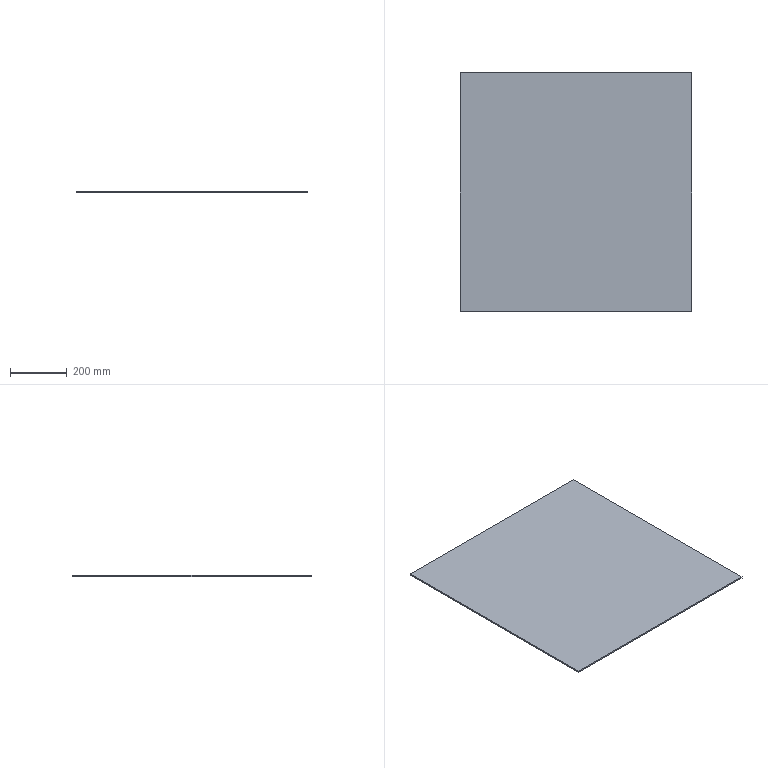Part | SolidWorks | features Extrusion 1, HoleWzd 1 | 1 solid | 6 faces | box 817 x 842 x 5 mm | volume 3439570 mm3 | plane 6
STEP:
#1=CARTESIAN_POINT('',(408.5,-421.,0.));
#2=VERTEX_POINT('',#1);
#3=CARTESIAN_POINT('',(408.5,421.,0.));
#4=VERTEX_POINT('',#3);
#5=CARTESIAN_POINT('',(408.5,421.,0.));
#6=DIRECTION('',(0.,1.,0.));
#7=VECTOR('',#6,1000.);
#8=LINE('',#5,#7);
#9=EDGE_CURVE('',#2,#4,#8,.T.);
#10=ORIENTED_EDGE('',*,*,#9,.T.);
#11=CARTESIAN_POINT('',(408.5,421.,5.));
#12=VERTEX_POINT('',#11);
#13=CARTESIAN_POINT('',(408.5,421.,5.));
#14=DIRECTION('',(0.,0.,-1.));
#15=VECTOR('',#14,1000.);
#16=LINE('',#13,#15);
#17=EDGE_CURVE('',#12,#4,#16,.T.);
#18=ORIENTED_EDGE('',*,*,#17,.F.);
#19=CARTESIAN_POINT('',(408.5,-421.,5.));
#20=VERTEX_POINT('',#19);
#21=CARTESIAN_POINT('',(408.5,421.,5.));
#22=DIRECTION('',(0.,1.,0.));
#23=VECTOR('',#22,1000.);
#24=LINE('',#21,#23);
#25=EDGE_CURVE('',#20,#12,#24,.T.);
#26=ORIENTED_EDGE('',*,*,#25,.F.);
#27=CARTESIAN_POINT('',(408.5,-421.,5.));
#28=DIRECTION('',(0.,0.,-1.));
#29=VECTOR('',#28,1000.);
#30=LINE('',#27,#29);
#31=EDGE_CURVE('',#20,#2,#30,.T.);
#32=ORIENTED_EDGE('',*,*,#31,.T.);
#33=EDGE_LOOP('',(#10,#18,#26,#32));
#34=FACE_OUTER_BOUND('',#33,.T.);
#35=CARTESIAN_POINT('',(408.5,421.,5.));
#36=DIRECTION('',(-1.,0.,0.));
#37=DIRECTION('',(0.,-1.,0.));
#38=AXIS2_PLACEMENT_3D('',#35,#36,#37);
#39=PLANE('',#38);
#40=ADVANCED_FACE('',(#34),#39,.F.);
#41=CARTESIAN_POINT('',(-408.5,421.,0.));
#42=VERTEX_POINT('',#41);
#43=CARTESIAN_POINT('',(-408.5,421.,0.));
#44=DIRECTION('',(-1.,0.,0.));
#45=VECTOR('',#44,1000.);
#46=LINE('',#43,#45);
#47=EDGE_CURVE('',#4,#42,#46,.T.);
#48=ORIENTED_EDGE('',*,*,#47,.T.);
#49=CARTESIAN_POINT('',(-408.5,421.,5.));
#50=VERTEX_POINT('',#49);
#51=CARTESIAN_POINT('',(-408.5,421.,5.));
#52=DIRECTION('',(0.,0.,-1.));
#53=VECTOR('',#52,1000.);
#54=LINE('',#51,#53);
#55=EDGE_CURVE('',#50,#42,#54,.T.);
#56=ORIENTED_EDGE('',*,*,#55,.F.);
#57=CARTESIAN_POINT('',(-408.5,421.,5.));
#58=DIRECTION('',(-1.,0.,0.));
#59=VECTOR('',#58,1000.);
#60=LINE('',#57,#59);
#61=EDGE_CURVE('',#12,#50,#60,.T.);
#62=ORIENTED_EDGE('',*,*,#61,.F.);
#63=ORIENTED_EDGE('',*,*,#17,.T.);
#64=EDGE_LOOP('',(#48,#56,#62,#63));
#65=FACE_OUTER_BOUND('',#64,.T.);
#66=CARTESIAN_POINT('',(-408.5,421.,5.));
#67=DIRECTION('',(0.,-1.,0.));
#68=DIRECTION('',(0.,0.,-1.));
#69=AXIS2_PLACEMENT_3D('',#66,#67,#68);
#70=PLANE('',#69);
#71=ADVANCED_FACE('',(#65),#70,.F.);
#72=CARTESIAN_POINT('',(-408.5,-421.,0.));
#73=VERTEX_POINT('',#72);
#74=CARTESIAN_POINT('',(-408.5,421.,0.));
#75=DIRECTION('',(0.,-1.,0.));
#76=VECTOR('',#75,1000.);
#77=LINE('',#74,#76);
#78=EDGE_CURVE('',#42,#73,#77,.T.);
#79=ORIENTED_EDGE('',*,*,#78,.T.);
#80=CARTESIAN_POINT('',(-408.5,-421.,5.));
#81=VERTEX_POINT('',#80);
#82=CARTESIAN_POINT('',(-408.5,-421.,5.));
#83=DIRECTION('',(0.,0.,-1.));
#84=VECTOR('',#83,1000.);
#85=LINE('',#82,#84);
#86=EDGE_CURVE('',#81,#73,#85,.T.);
#87=ORIENTED_EDGE('',*,*,#86,.F.);
#88=CARTESIAN_POINT('',(-408.5,421.,5.));
#89=DIRECTION('',(0.,-1.,0.));
#90=VECTOR('',#89,1000.);
#91=LINE('',#88,#90);
#92=EDGE_CURVE('',#50,#81,#91,.T.);
#93=ORIENTED_EDGE('',*,*,#92,.F.);
#94=ORIENTED_EDGE('',*,*,#55,.T.);
#95=EDGE_LOOP('',(#79,#87,#93,#94));
#96=FACE_OUTER_BOUND('',#95,.T.);
#97=CARTESIAN_POINT('',(-408.5,421.,5.));
#98=DIRECTION('',(1.,0.,0.));
#99=DIRECTION('',(0.,1.,0.));
#100=AXIS2_PLACEMENT_3D('',#97,#98,#99);
#101=PLANE('',#100);
#102=ADVANCED_FACE('',(#96),#101,.F.);
#103=CARTESIAN_POINT('',(-408.5,-421.,0.));
#104=DIRECTION('',(1.,0.,0.));
#105=VECTOR('',#104,1000.);
#106=LINE('',#103,#105);
#107=EDGE_CURVE('',#73,#2,#106,.T.);
#108=ORIENTED_EDGE('',*,*,#107,.T.);
#109=ORIENTED_EDGE('',*,*,#31,.F.);
#110=CARTESIAN_POINT('',(-408.5,-421.,5.));
#111=DIRECTION('',(1.,0.,0.));
#112=VECTOR('',#111,1000.);
#113=LINE('',#110,#112);
#114=EDGE_CURVE('',#81,#20,#113,.T.);
#115=ORIENTED_EDGE('',*,*,#114,.F.);
#116=ORIENTED_EDGE('',*,*,#86,.T.);
#117=EDGE_LOOP('',(#108,#109,#115,#116));
#118=FACE_OUTER_BOUND('',#117,.T.);
#119=CARTESIAN_POINT('',(-408.5,-421.,5.));
#120=DIRECTION('',(0.,1.,0.));
#121=DIRECTION('',(0.,0.,1.));
#122=AXIS2_PLACEMENT_3D('',#119,#120,#121);
#123=PLANE('',#122);
#124=ADVANCED_FACE('',(#118),#123,.F.);
#125=ORIENTED_EDGE('',*,*,#25,.T.);
#126=ORIENTED_EDGE('',*,*,#61,.T.);
#127=ORIENTED_EDGE('',*,*,#92,.T.);
#128=ORIENTED_EDGE('',*,*,#114,.T.);
#129=EDGE_LOOP('',(#125,#126,#127,#128));
#130=FACE_OUTER_BOUND('',#129,.T.);
#131=CARTESIAN_POINT('',(0.,0.,5.));
#132=DIRECTION('',(0.,0.,1.));
#133=DIRECTION('',(1.,0.,0.));
#134=AXIS2_PLACEMENT_3D('',#131,#132,#133);
#135=PLANE('',#134);
#136=ADVANCED_FACE('',(#130),#135,.T.);
#137=ORIENTED_EDGE('',*,*,#9,.F.);
#138=ORIENTED_EDGE('',*,*,#107,.F.);
#139=ORIENTED_EDGE('',*,*,#78,.F.);
#140=ORIENTED_EDGE('',*,*,#47,.F.);
#141=EDGE_LOOP('',(#137,#138,#139,#140));
#142=FACE_OUTER_BOUND('',#141,.T.);
#143=CARTESIAN_POINT('',(0.,0.,0.));
#144=DIRECTION('',(0.,0.,1.));
#145=DIRECTION('',(1.,0.,0.));
#146=AXIS2_PLACEMENT_3D('',#143,#144,#145);
#147=PLANE('',#146);
#148=ADVANCED_FACE('',(#142),#147,.F.);
#149=CLOSED_SHELL('',(#40,#71,#102,#124,#136,#148));
#150=MANIFOLD_SOLID_BREP('',#149);
#151=CARTESIAN_POINT('',(0.,0.,0.));
#152=DIRECTION('',(0.,0.,1.));
#153=DIRECTION('',(1.,0.,0.));
#154=AXIS2_PLACEMENT_3D('',#151,#152,#153);
#155=(LENGTH_UNIT()NAMED_UNIT(*)SI_UNIT(.MILLI.,.METRE.));
#156=UNCERTAINTY_MEASURE_WITH_UNIT(LENGTH_MEASURE(0.00001),#155,'','');
#157=(NAMED_UNIT(*)PLANE_ANGLE_UNIT()SI_UNIT($,.RADIAN.));
#158=(NAMED_UNIT(*)SI_UNIT($,.STERADIAN.)SOLID_ANGLE_UNIT());
#159=(GEOMETRIC_REPRESENTATION_CONTEXT(3)GLOBAL_UNCERTAINTY_ASSIGNED_CONTEXT((#156))GLOBAL_UNIT_ASSIGNED_CONTEXT((#155,#157,#158))REPRESENTATION_CONTEXT('',''));
#160=ADVANCED_BREP_SHAPE_REPRESENTATION('',(#150,#154),#159);